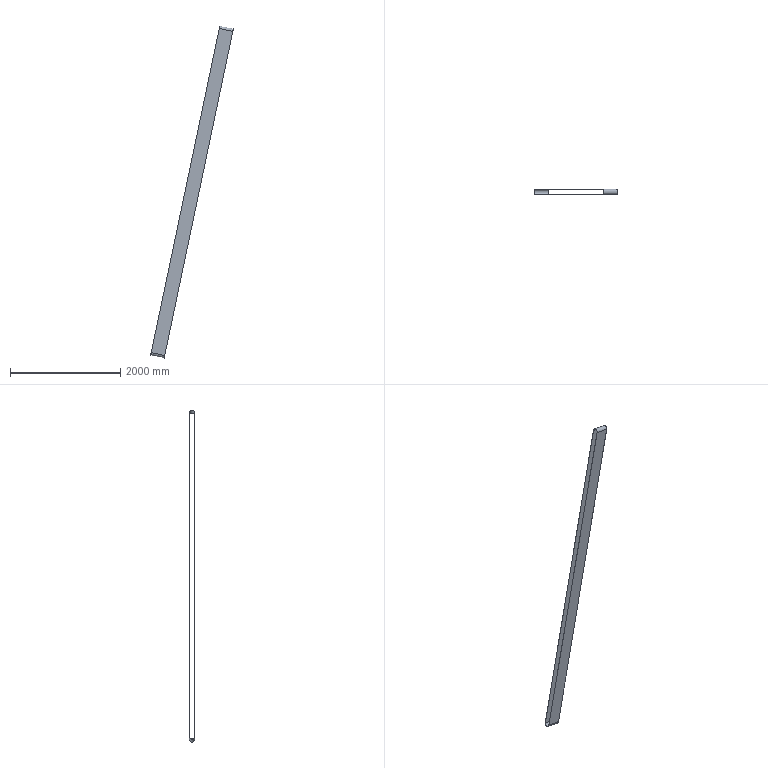Part | STEP file | ESTEIRA_003 | 1 solid | 10 faces | box 1498 x 95 x 6016 mm | volume 6146084 mm3 | plane 6 | cylinder 4 | commonest cylinder face diameters 91 x2 95 x2
STEP:
#1=CARTESIAN_POINT('',(0.,0.,0.));
#2=DIRECTION('',(0.,0.,1.));
#3=DIRECTION('',(1.,0.,0.));
#4=AXIS2_PLACEMENT_3D('',#1,#2,#3);
#5=CARTESIAN_POINT('',(-4261.561,-580.65,1712.598));
#6=VERTEX_POINT('',#5);
#7=CARTESIAN_POINT('',(-4506.218,-580.65,1764.008));
#8=VERTEX_POINT('',#7);
#9=CARTESIAN_POINT('',(-4261.561,-580.65,1712.598));
#10=DIRECTION('',(-0.9786,0.,0.2056));
#11=VECTOR('',#10,1.);
#12=LINE('',#9,#11);
#13=CARTESIAN_POINT('',(-4383.89,-580.65,1738.303));
#14=DIRECTION('',(0.,1.,0.));
#15=DIRECTION('',(0.,0.,1.));
#16=AXIS2_PLACEMENT_3D('',#13,#14,#15);
#17=PLANE('',#16);
#18=CARTESIAN_POINT('',(-25.705,122.328));
#19=DIRECTION('',(0.2056,-0.9786));
#20=VECTOR('',#19,1.);
#21=LINE('',#18,#20);
#22=(GEOMETRIC_REPRESENTATION_CONTEXT(2)PARAMETRIC_REPRESENTATION_CONTEXT()REPRESENTATION_CONTEXT('',''));
#23=DEFINITIONAL_REPRESENTATION('',(#21),#22);
#24=PCURVE('',#17,#23);
#25=CARTESIAN_POINT('',(-4383.89,-628.15,1738.303));
#26=DIRECTION('',(0.9786,0.,-0.2056));
#27=DIRECTION('',(0.,1.,0.));
#28=AXIS2_PLACEMENT_3D('',#25,#26,#27);
#29=CYLINDRICAL_SURFACE('',#28,47.5);
#30=CARTESIAN_POINT('',(0.,125.));
#31=DIRECTION('',(0.,-1.));
#32=VECTOR('',#31,1.);
#33=LINE('',#30,#32);
#34=(GEOMETRIC_REPRESENTATION_CONTEXT(2)PARAMETRIC_REPRESENTATION_CONTEXT()REPRESENTATION_CONTEXT('',''));
#35=DEFINITIONAL_REPRESENTATION('',(#33),#34);
#36=PCURVE('',#29,#35);
#37=SURFACE_CURVE('',#12,(#24,#36),.PCURVE_S1.);
#38=EDGE_CURVE('',#6,#8,#37,.T.);
#39=ORIENTED_EDGE('',*,*,#38,.F.);
#40=CARTESIAN_POINT('',(-5495.421,-580.65,-4159.165));
#41=VERTEX_POINT('',#40);
#42=CARTESIAN_POINT('',(-4261.561,-580.65,1712.598));
#43=DIRECTION('',(-0.2056,0.,-0.9786));
#44=VECTOR('',#43,1.);
#45=LINE('',#42,#44);
#46=CARTESIAN_POINT('',(-25.705,122.328));
#47=DIRECTION('',(-0.9786,-0.2056));
#48=VECTOR('',#47,1.);
#49=LINE('',#46,#48);
#50=(GEOMETRIC_REPRESENTATION_CONTEXT(2)PARAMETRIC_REPRESENTATION_CONTEXT()REPRESENTATION_CONTEXT('',''));
#51=DEFINITIONAL_REPRESENTATION('',(#49),#50);
#52=PCURVE('',#17,#51);
#53=CARTESIAN_POINT('',(-4426.,0.,930.055));
#54=DIRECTION('',(0.9786,0.,-0.2056));
#55=DIRECTION('',(-0.2056,0.,-0.9786));
#56=AXIS2_PLACEMENT_3D('',#53,#54,#55);
#57=PLANE('',#56);
#58=CARTESIAN_POINT('',(-799.633,-580.65));
#59=DIRECTION('',(1.,0.));
#60=VECTOR('',#59,1.);
#61=LINE('',#58,#60);
#62=(GEOMETRIC_REPRESENTATION_CONTEXT(2)PARAMETRIC_REPRESENTATION_CONTEXT()REPRESENTATION_CONTEXT('',''));
#63=DEFINITIONAL_REPRESENTATION('',(#61),#62);
#64=PCURVE('',#57,#63);
#65=SURFACE_CURVE('',#45,(#52,#64),.PCURVE_S1.);
#66=EDGE_CURVE('',#6,#41,#65,.T.);
#67=ORIENTED_EDGE('',*,*,#66,.T.);
#68=CARTESIAN_POINT('',(-5740.078,-580.65,-4107.754));
#69=VERTEX_POINT('',#68);
#70=CARTESIAN_POINT('',(-5495.421,-580.65,-4159.165));
#71=DIRECTION('',(-0.9786,0.,0.2056));
#72=VECTOR('',#71,1.);
#73=LINE('',#70,#72);
#74=CARTESIAN_POINT('',(-5897.468,-1111.531));
#75=DIRECTION('',(0.2056,-0.9786));
#76=VECTOR('',#75,1.);
#77=LINE('',#74,#76);
#78=(GEOMETRIC_REPRESENTATION_CONTEXT(2)PARAMETRIC_REPRESENTATION_CONTEXT()REPRESENTATION_CONTEXT('',''));
#79=DEFINITIONAL_REPRESENTATION('',(#77),#78);
#80=PCURVE('',#17,#79);
#81=CARTESIAN_POINT('',(-5617.749,-628.15,-4133.459));
#82=DIRECTION('',(0.9786,0.,-0.2056));
#83=DIRECTION('',(0.,-1.,0.));
#84=AXIS2_PLACEMENT_3D('',#81,#82,#83);
#85=CYLINDRICAL_SURFACE('',#84,47.5);
#86=CARTESIAN_POINT('',(3.142,125.));
#87=DIRECTION('',(0.,-1.));
#88=VECTOR('',#87,1.);
#89=LINE('',#86,#88);
#90=(GEOMETRIC_REPRESENTATION_CONTEXT(2)PARAMETRIC_REPRESENTATION_CONTEXT()REPRESENTATION_CONTEXT('',''));
#91=DEFINITIONAL_REPRESENTATION('',(#89),#90);
#92=PCURVE('',#85,#91);
#93=SURFACE_CURVE('',#73,(#80,#92),.PCURVE_S1.);
#94=EDGE_CURVE('',#41,#69,#93,.T.);
#95=ORIENTED_EDGE('',*,*,#94,.T.);
#96=CARTESIAN_POINT('',(-4506.218,-580.65,1764.008));
#97=DIRECTION('',(-0.2056,0.,-0.9786));
#98=VECTOR('',#97,1.);
#99=LINE('',#96,#98);
#100=CARTESIAN_POINT('',(25.705,-122.328));
#101=DIRECTION('',(-0.9786,-0.2056));
#102=VECTOR('',#101,1.);
#103=LINE('',#100,#102);
#104=(GEOMETRIC_REPRESENTATION_CONTEXT(2)PARAMETRIC_REPRESENTATION_CONTEXT()REPRESENTATION_CONTEXT('',''));
#105=DEFINITIONAL_REPRESENTATION('',(#103),#104);
#106=PCURVE('',#17,#105);
#107=CARTESIAN_POINT('',(-4670.657,0.,981.466));
#108=DIRECTION('',(0.9786,0.,-0.2056));
#109=DIRECTION('',(-0.2056,0.,-0.9786));
#110=AXIS2_PLACEMENT_3D('',#107,#108,#109);
#111=PLANE('',#110);
#112=CARTESIAN_POINT('',(-799.633,-580.65));
#113=DIRECTION('',(1.,0.));
#114=VECTOR('',#113,1.);
#115=LINE('',#112,#114);
#116=(GEOMETRIC_REPRESENTATION_CONTEXT(2)PARAMETRIC_REPRESENTATION_CONTEXT()REPRESENTATION_CONTEXT('',''));
#117=DEFINITIONAL_REPRESENTATION('',(#115),#116);
#118=PCURVE('',#111,#117);
#119=SURFACE_CURVE('',#99,(#106,#118),.PCURVE_S1.);
#120=EDGE_CURVE('',#8,#69,#119,.T.);
#121=ORIENTED_EDGE('',*,*,#120,.F.);
#122=EDGE_LOOP('',(#39,#67,#95,#121));
#123=FACE_BOUND('',#122,.T.);
#124=ADVANCED_FACE('',(#123),#17,.T.);
#125=CARTESIAN_POINT('',(-4506.218,-675.65,1764.008));
#126=VERTEX_POINT('',#125);
#127=CARTESIAN_POINT('',(-4506.218,-628.15,1764.008));
#128=DIRECTION('',(0.9786,0.,-0.2056));
#129=DIRECTION('',(0.2056,0.,0.9786));
#130=AXIS2_PLACEMENT_3D('',#127,#128,#129);
#131=CIRCLE('',#130,47.5);
#132=CARTESIAN_POINT('',(-4.712,-125.));
#133=DIRECTION('',(1.,0.));
#134=VECTOR('',#133,1.);
#135=LINE('',#132,#134);
#136=(GEOMETRIC_REPRESENTATION_CONTEXT(2)PARAMETRIC_REPRESENTATION_CONTEXT()REPRESENTATION_CONTEXT('',''));
#137=DEFINITIONAL_REPRESENTATION('',(#135),#136);
#138=PCURVE('',#29,#137);
#139=CARTESIAN_POINT('',(-799.633,-628.15));
#140=DIRECTION('',(-1.,0.));
#141=AXIS2_PLACEMENT_2D('',#139,#140);
#142=CIRCLE('',#141,47.5);
#143=(GEOMETRIC_REPRESENTATION_CONTEXT(2)PARAMETRIC_REPRESENTATION_CONTEXT()REPRESENTATION_CONTEXT('',''));
#144=DEFINITIONAL_REPRESENTATION('',(#142),#143);
#145=PCURVE('',#111,#144);
#146=SURFACE_CURVE('',#131,(#138,#145),.PCURVE_S1.);
#147=EDGE_CURVE('',#8,#126,#146,.T.);
#148=ORIENTED_EDGE('',*,*,#147,.T.);
#149=CARTESIAN_POINT('',(-4261.561,-675.65,1712.598));
#150=VERTEX_POINT('',#149);
#151=CARTESIAN_POINT('',(-4506.218,-675.65,1764.008));
#152=DIRECTION('',(0.9786,0.,-0.2056));
#153=VECTOR('',#152,1.);
#154=LINE('',#151,#153);
#155=CARTESIAN_POINT('',(3.142,-125.));
#156=DIRECTION('',(0.,1.));
#157=VECTOR('',#156,1.);
#158=LINE('',#155,#157);
#159=(GEOMETRIC_REPRESENTATION_CONTEXT(2)PARAMETRIC_REPRESENTATION_CONTEXT()REPRESENTATION_CONTEXT('',''));
#160=DEFINITIONAL_REPRESENTATION('',(#158),#159);
#161=PCURVE('',#29,#160);
#162=CARTESIAN_POINT('',(-5617.749,-675.65,-4133.459));
#163=DIRECTION('',(0.,-1.,0.));
#164=DIRECTION('',(0.,0.,-1.));
#165=AXIS2_PLACEMENT_3D('',#162,#163,#164);
#166=PLANE('',#165);
#167=CARTESIAN_POINT('',(-5897.468,1111.531));
#168=DIRECTION('',(0.2056,0.9786));
#169=VECTOR('',#168,1.);
#170=LINE('',#167,#169);
#171=(GEOMETRIC_REPRESENTATION_CONTEXT(2)PARAMETRIC_REPRESENTATION_CONTEXT()REPRESENTATION_CONTEXT('',''));
#172=DEFINITIONAL_REPRESENTATION('',(#170),#171);
#173=PCURVE('',#166,#172);
#174=SURFACE_CURVE('',#154,(#161,#173),.PCURVE_S1.);
#175=EDGE_CURVE('',#126,#150,#174,.T.);
#176=ORIENTED_EDGE('',*,*,#175,.T.);
#177=CARTESIAN_POINT('',(-4261.561,-628.15,1712.598));
#178=DIRECTION('',(0.9786,0.,-0.2056));
#179=DIRECTION('',(0.2056,0.,0.9786));
#180=AXIS2_PLACEMENT_3D('',#177,#178,#179);
#181=CIRCLE('',#180,47.5);
#182=CARTESIAN_POINT('',(-4.712,125.));
#183=DIRECTION('',(1.,0.));
#184=VECTOR('',#183,1.);
#185=LINE('',#182,#184);
#186=(GEOMETRIC_REPRESENTATION_CONTEXT(2)PARAMETRIC_REPRESENTATION_CONTEXT()REPRESENTATION_CONTEXT('',''));
#187=DEFINITIONAL_REPRESENTATION('',(#185),#186);
#188=PCURVE('',#29,#187);
#189=CARTESIAN_POINT('',(-799.633,-628.15));
#190=DIRECTION('',(-1.,0.));
#191=AXIS2_PLACEMENT_2D('',#189,#190);
#192=CIRCLE('',#191,47.5);
#193=(GEOMETRIC_REPRESENTATION_CONTEXT(2)PARAMETRIC_REPRESENTATION_CONTEXT()REPRESENTATION_CONTEXT('',''));
#194=DEFINITIONAL_REPRESENTATION('',(#192),#193);
#195=PCURVE('',#57,#194);
#196=SURFACE_CURVE('',#181,(#188,#195),.PCURVE_S1.);
#197=EDGE_CURVE('',#6,#150,#196,.T.);
#198=ORIENTED_EDGE('',*,*,#197,.F.);
#199=ORIENTED_EDGE('',*,*,#38,.T.);
#200=EDGE_LOOP('',(#148,#176,#198,#199));
#201=FACE_BOUND('',#200,.T.);
#202=ADVANCED_FACE('',(#201),#29,.T.);
#203=CARTESIAN_POINT('',(-5495.421,-675.65,-4159.165));
#204=VERTEX_POINT('',#203);
#205=CARTESIAN_POINT('',(-5740.078,-675.65,-4107.754));
#206=VERTEX_POINT('',#205);
#207=CARTESIAN_POINT('',(-5495.421,-675.65,-4159.165));
#208=DIRECTION('',(-0.9786,0.,0.2056));
#209=VECTOR('',#208,1.);
#210=LINE('',#207,#209);
#211=CARTESIAN_POINT('',(25.705,122.328));
#212=DIRECTION('',(-0.2056,-0.9786));
#213=VECTOR('',#212,1.);
#214=LINE('',#211,#213);
#215=(GEOMETRIC_REPRESENTATION_CONTEXT(2)PARAMETRIC_REPRESENTATION_CONTEXT()REPRESENTATION_CONTEXT('',''));
#216=DEFINITIONAL_REPRESENTATION('',(#214),#215);
#217=PCURVE('',#166,#216);
#218=CARTESIAN_POINT('',(0.,125.));
#219=DIRECTION('',(0.,-1.));
#220=VECTOR('',#219,1.);
#221=LINE('',#218,#220);
#222=(GEOMETRIC_REPRESENTATION_CONTEXT(2)PARAMETRIC_REPRESENTATION_CONTEXT()REPRESENTATION_CONTEXT('',''));
#223=DEFINITIONAL_REPRESENTATION('',(#221),#222);
#224=PCURVE('',#85,#223);
#225=SURFACE_CURVE('',#210,(#217,#224),.PCURVE_S1.);
#226=EDGE_CURVE('',#204,#206,#225,.T.);
#227=ORIENTED_EDGE('',*,*,#226,.F.);
#228=CARTESIAN_POINT('',(-5495.421,-675.65,-4159.165));
#229=DIRECTION('',(0.2056,0.,0.9786));
#230=VECTOR('',#229,1.);
#231=LINE('',#228,#230);
#232=CARTESIAN_POINT('',(25.705,122.328));
#233=DIRECTION('',(-0.9786,0.2056));
#234=VECTOR('',#233,1.);
#235=LINE('',#232,#234);
#236=(GEOMETRIC_REPRESENTATION_CONTEXT(2)PARAMETRIC_REPRESENTATION_CONTEXT()REPRESENTATION_CONTEXT('',''));
#237=DEFINITIONAL_REPRESENTATION('',(#235),#236);
#238=PCURVE('',#166,#237);
#239=CARTESIAN_POINT('',(5200.367,-675.65));
#240=DIRECTION('',(-1.,0.));
#241=VECTOR('',#240,1.);
#242=LINE('',#239,#241);
#243=(GEOMETRIC_REPRESENTATION_CONTEXT(2)PARAMETRIC_REPRESENTATION_CONTEXT()REPRESENTATION_CONTEXT('',''));
#244=DEFINITIONAL_REPRESENTATION('',(#242),#243);
#245=PCURVE('',#57,#244);
#246=SURFACE_CURVE('',#231,(#238,#245),.PCURVE_S1.);
#247=EDGE_CURVE('',#204,#150,#246,.T.);
#248=ORIENTED_EDGE('',*,*,#247,.T.);
#249=ORIENTED_EDGE('',*,*,#175,.F.);
#250=CARTESIAN_POINT('',(-5740.078,-675.65,-4107.754));
#251=DIRECTION('',(0.2056,0.,0.9786));
#252=VECTOR('',#251,1.);
#253=LINE('',#250,#252);
#254=CARTESIAN_POINT('',(-25.705,-122.328));
#255=DIRECTION('',(-0.9786,0.2056));
#256=VECTOR('',#255,1.);
#257=LINE('',#254,#256);
#258=(GEOMETRIC_REPRESENTATION_CONTEXT(2)PARAMETRIC_REPRESENTATION_CONTEXT()REPRESENTATION_CONTEXT('',''));
#259=DEFINITIONAL_REPRESENTATION('',(#257),#258);
#260=PCURVE('',#166,#259);
#261=CARTESIAN_POINT('',(5200.367,-675.65));
#262=DIRECTION('',(-1.,0.));
#263=VECTOR('',#262,1.);
#264=LINE('',#261,#263);
#265=(GEOMETRIC_REPRESENTATION_CONTEXT(2)PARAMETRIC_REPRESENTATION_CONTEXT()REPRESENTATION_CONTEXT('',''));
#266=DEFINITIONAL_REPRESENTATION('',(#264),#265);
#267=PCURVE('',#111,#266);
#268=SURFACE_CURVE('',#253,(#260,#267),.PCURVE_S1.);
#269=EDGE_CURVE('',#206,#126,#268,.T.);
#270=ORIENTED_EDGE('',*,*,#269,.F.);
#271=EDGE_LOOP('',(#227,#248,#249,#270));
#272=FACE_BOUND('',#271,.T.);
#273=ADVANCED_FACE('',(#272),#166,.T.);
#274=CARTESIAN_POINT('',(-5740.078,-628.15,-4107.754));
#275=DIRECTION('',(0.9786,0.,-0.2056));
#276=DIRECTION('',(0.2056,0.,0.9786));
#277=AXIS2_PLACEMENT_3D('',#274,#275,#276);
#278=CIRCLE('',#277,47.5);
#279=CARTESIAN_POINT('',(-1.571,-125.));
#280=DIRECTION('',(1.,0.));
#281=VECTOR('',#280,1.);
#282=LINE('',#279,#281);
#283=(GEOMETRIC_REPRESENTATION_CONTEXT(2)PARAMETRIC_REPRESENTATION_CONTEXT()REPRESENTATION_CONTEXT('',''));
#284=DEFINITIONAL_REPRESENTATION('',(#282),#283);
#285=PCURVE('',#85,#284);
#286=CARTESIAN_POINT('',(5200.367,-628.15));
#287=DIRECTION('',(-1.,0.));
#288=AXIS2_PLACEMENT_2D('',#286,#287);
#289=CIRCLE('',#288,47.5);
#290=(GEOMETRIC_REPRESENTATION_CONTEXT(2)PARAMETRIC_REPRESENTATION_CONTEXT()REPRESENTATION_CONTEXT('',''));
#291=DEFINITIONAL_REPRESENTATION('',(#289),#290);
#292=PCURVE('',#111,#291);
#293=SURFACE_CURVE('',#278,(#285,#292),.PCURVE_S1.);
#294=EDGE_CURVE('',#206,#69,#293,.T.);
#295=ORIENTED_EDGE('',*,*,#294,.T.);
#296=ORIENTED_EDGE('',*,*,#94,.F.);
#297=CARTESIAN_POINT('',(-5495.421,-628.15,-4159.165));
#298=DIRECTION('',(0.9786,0.,-0.2056));
#299=DIRECTION('',(0.2056,0.,0.9786));
#300=AXIS2_PLACEMENT_3D('',#297,#298,#299);
#301=CIRCLE('',#300,47.5);
#302=CARTESIAN_POINT('',(-1.571,125.));
#303=DIRECTION('',(1.,0.));
#304=VECTOR('',#303,1.);
#305=LINE('',#302,#304);
#306=(GEOMETRIC_REPRESENTATION_CONTEXT(2)PARAMETRIC_REPRESENTATION_CONTEXT()REPRESENTATION_CONTEXT('',''));
#307=DEFINITIONAL_REPRESENTATION('',(#305),#306);
#308=PCURVE('',#85,#307);
#309=CARTESIAN_POINT('',(5200.367,-628.15));
#310=DIRECTION('',(-1.,0.));
#311=AXIS2_PLACEMENT_2D('',#309,#310);
#312=CIRCLE('',#311,47.5);
#313=(GEOMETRIC_REPRESENTATION_CONTEXT(2)PARAMETRIC_REPRESENTATION_CONTEXT()REPRESENTATION_CONTEXT('',''));
#314=DEFINITIONAL_REPRESENTATION('',(#312),#313);
#315=PCURVE('',#57,#314);
#316=SURFACE_CURVE('',#301,(#308,#315),.PCURVE_S1.);
#317=EDGE_CURVE('',#204,#41,#316,.T.);
#318=ORIENTED_EDGE('',*,*,#317,.F.);
#319=ORIENTED_EDGE('',*,*,#226,.T.);
#320=EDGE_LOOP('',(#295,#296,#318,#319));
#321=FACE_BOUND('',#320,.T.);
#322=ADVANCED_FACE('',(#321),#85,.T.);
#323=CARTESIAN_POINT('',(-4506.218,-582.65,1764.008));
#324=VERTEX_POINT('',#323);
#325=CARTESIAN_POINT('',(-5740.078,-582.65,-4107.754));
#326=VERTEX_POINT('',#325);
#327=CARTESIAN_POINT('',(-4506.218,-582.65,1764.008));
#328=DIRECTION('',(-0.2056,0.,-0.9786));
#329=VECTOR('',#328,1.);
#330=LINE('',#327,#329);
#331=CARTESIAN_POINT('',(-4383.89,-582.65,1738.303));
#332=DIRECTION('',(0.,1.,0.));
#333=DIRECTION('',(0.,0.,1.));
#334=AXIS2_PLACEMENT_3D('',#331,#332,#333);
#335=PLANE('',#334);
#336=CARTESIAN_POINT('',(25.705,-122.328));
#337=DIRECTION('',(-0.9786,-0.2056));
#338=VECTOR('',#337,1.);
#339=LINE('',#336,#338);
#340=(GEOMETRIC_REPRESENTATION_CONTEXT(2)PARAMETRIC_REPRESENTATION_CONTEXT()REPRESENTATION_CONTEXT('',''));
#341=DEFINITIONAL_REPRESENTATION('',(#339),#340);
#342=PCURVE('',#335,#341);
#343=CARTESIAN_POINT('',(-799.633,-582.65));
#344=DIRECTION('',(1.,0.));
#345=VECTOR('',#344,1.);
#346=LINE('',#343,#345);
#347=(GEOMETRIC_REPRESENTATION_CONTEXT(2)PARAMETRIC_REPRESENTATION_CONTEXT()REPRESENTATION_CONTEXT('',''));
#348=DEFINITIONAL_REPRESENTATION('',(#346),#347);
#349=PCURVE('',#111,#348);
#350=SURFACE_CURVE('',#330,(#342,#349),.PCURVE_S1.);
#351=EDGE_CURVE('',#324,#326,#350,.T.);
#352=ORIENTED_EDGE('',*,*,#351,.T.);
#353=CARTESIAN_POINT('',(-5495.421,-582.65,-4159.165));
#354=VERTEX_POINT('',#353);
#355=CARTESIAN_POINT('',(-5495.421,-582.65,-4159.165));
#356=DIRECTION('',(-0.9786,0.,0.2056));
#357=VECTOR('',#356,1.);
#358=LINE('',#355,#357);
#359=CARTESIAN_POINT('',(-5897.468,-1111.531));
#360=DIRECTION('',(0.2056,-0.9786));
#361=VECTOR('',#360,1.);
#362=LINE('',#359,#361);
#363=(GEOMETRIC_REPRESENTATION_CONTEXT(2)PARAMETRIC_REPRESENTATION_CONTEXT()REPRESENTATION_CONTEXT('',''));
#364=DEFINITIONAL_REPRESENTATION('',(#362),#363);
#365=PCURVE('',#335,#364);
#366=CARTESIAN_POINT('',(-5617.749,-628.15,-4133.459));
#367=DIRECTION('',(0.9786,0.,-0.2056));
#368=DIRECTION('',(0.,-1.,0.));
#369=AXIS2_PLACEMENT_3D('',#366,#367,#368);
#370=CYLINDRICAL_SURFACE('',#369,45.5);
#371=CARTESIAN_POINT('',(3.142,125.));
#372=DIRECTION('',(0.,-1.));
#373=VECTOR('',#372,1.);
#374=LINE('',#371,#373);
#375=(GEOMETRIC_REPRESENTATION_CONTEXT(2)PARAMETRIC_REPRESENTATION_CONTEXT()REPRESENTATION_CONTEXT('',''));
#376=DEFINITIONAL_REPRESENTATION('',(#374),#375);
#377=PCURVE('',#370,#376);
#378=SURFACE_CURVE('',#358,(#365,#377),.PCURVE_S1.);
#379=EDGE_CURVE('',#354,#326,#378,.T.);
#380=ORIENTED_EDGE('',*,*,#379,.F.);
#381=CARTESIAN_POINT('',(-4261.561,-582.65,1712.598));
#382=VERTEX_POINT('',#381);
#383=CARTESIAN_POINT('',(-4261.561,-582.65,1712.598));
#384=DIRECTION('',(-0.2056,0.,-0.9786));
#385=VECTOR('',#384,1.);
#386=LINE('',#383,#385);
#387=CARTESIAN_POINT('',(-25.705,122.328));
#388=DIRECTION('',(-0.9786,-0.2056));
#389=VECTOR('',#388,1.);
#390=LINE('',#387,#389);
#391=(GEOMETRIC_REPRESENTATION_CONTEXT(2)PARAMETRIC_REPRESENTATION_CONTEXT()REPRESENTATION_CONTEXT('',''));
#392=DEFINITIONAL_REPRESENTATION('',(#390),#391);
#393=PCURVE('',#335,#392);
#394=CARTESIAN_POINT('',(-799.633,-582.65));
#395=DIRECTION('',(1.,0.));
#396=VECTOR('',#395,1.);
#397=LINE('',#394,#396);
#398=(GEOMETRIC_REPRESENTATION_CONTEXT(2)PARAMETRIC_REPRESENTATION_CONTEXT()REPRESENTATION_CONTEXT('',''));
#399=DEFINITIONAL_REPRESENTATION('',(#397),#398);
#400=PCURVE('',#57,#399);
#401=SURFACE_CURVE('',#386,(#393,#400),.PCURVE_S1.);
#402=EDGE_CURVE('',#382,#354,#401,.T.);
#403=ORIENTED_EDGE('',*,*,#402,.F.);
#404=CARTESIAN_POINT('',(-4261.561,-582.65,1712.598));
#405=DIRECTION('',(-0.9786,0.,0.2056));
#406=VECTOR('',#405,1.);
#407=LINE('',#404,#406);
#408=CARTESIAN_POINT('',(-25.705,122.328));
#409=DIRECTION('',(0.2056,-0.9786));
#410=VECTOR('',#409,1.);
#411=LINE('',#408,#410);
#412=(GEOMETRIC_REPRESENTATION_CONTEXT(2)PARAMETRIC_REPRESENTATION_CONTEXT()REPRESENTATION_CONTEXT('',''));
#413=DEFINITIONAL_REPRESENTATION('',(#411),#412);
#414=PCURVE('',#335,#413);
#415=CARTESIAN_POINT('',(-4383.89,-628.15,1738.303));
#416=DIRECTION('',(0.9786,0.,-0.2056));
#417=DIRECTION('',(0.,1.,0.));
#418=AXIS2_PLACEMENT_3D('',#415,#416,#417);
#419=CYLINDRICAL_SURFACE('',#418,45.5);
#420=CARTESIAN_POINT('',(0.,125.));
#421=DIRECTION('',(0.,-1.));
#422=VECTOR('',#421,1.);
#423=LINE('',#420,#422);
#424=(GEOMETRIC_REPRESENTATION_CONTEXT(2)PARAMETRIC_REPRESENTATION_CONTEXT()REPRESENTATION_CONTEXT('',''));
#425=DEFINITIONAL_REPRESENTATION('',(#423),#424);
#426=PCURVE('',#419,#425);
#427=SURFACE_CURVE('',#407,(#414,#426),.PCURVE_S1.);
#428=EDGE_CURVE('',#382,#324,#427,.T.);
#429=ORIENTED_EDGE('',*,*,#428,.T.);
#430=EDGE_LOOP('',(#352,#380,#403,#429));
#431=FACE_BOUND('',#430,.T.);
#432=ADVANCED_FACE('',(#431),#335,.F.);
#433=CARTESIAN_POINT('',(-5740.078,-673.65,-4107.754));
#434=VERTEX_POINT('',#433);
#435=CARTESIAN_POINT('',(-5740.078,-628.15,-4107.754));
#436=DIRECTION('',(0.9786,0.,-0.2056));
#437=DIRECTION('',(0.2056,0.,0.9786));
#438=AXIS2_PLACEMENT_3D('',#435,#436,#437);
#439=CIRCLE('',#438,45.5);
#440=CARTESIAN_POINT('',(-1.571,-125.));
#441=DIRECTION('',(1.,0.));
#442=VECTOR('',#441,1.);
#443=LINE('',#440,#442);
#444=(GEOMETRIC_REPRESENTATION_CONTEXT(2)PARAMETRIC_REPRESENTATION_CONTEXT()REPRESENTATION_CONTEXT('',''));
#445=DEFINITIONAL_REPRESENTATION('',(#443),#444);
#446=PCURVE('',#370,#445);
#447=CARTESIAN_POINT('',(5200.367,-628.15));
#448=DIRECTION('',(-1.,0.));
#449=AXIS2_PLACEMENT_2D('',#447,#448);
#450=CIRCLE('',#449,45.5);
#451=(GEOMETRIC_REPRESENTATION_CONTEXT(2)PARAMETRIC_REPRESENTATION_CONTEXT()REPRESENTATION_CONTEXT('',''));
#452=DEFINITIONAL_REPRESENTATION('',(#450),#451);
#453=PCURVE('',#111,#452);
#454=SURFACE_CURVE('',#439,(#446,#453),.PCURVE_S1.);
#455=EDGE_CURVE('',#434,#326,#454,.T.);
#456=ORIENTED_EDGE('',*,*,#455,.T.);
#457=ORIENTED_EDGE('',*,*,#379,.F.);
#458=CARTESIAN_POINT('',(-5495.421,-673.65,-4159.165));
#459=VERTEX_POINT('',#458);
#460=CARTESIAN_POINT('',(-5495.421,-628.15,-4159.165));
#461=DIRECTION('',(0.9786,0.,-0.2056));
#462=DIRECTION('',(0.2056,0.,0.9786));
#463=AXIS2_PLACEMENT_3D('',#460,#461,#462);
#464=CIRCLE('',#463,45.5);
#465=CARTESIAN_POINT('',(-1.571,125.));
#466=DIRECTION('',(1.,0.));
#467=VECTOR('',#466,1.);
#468=LINE('',#465,#467);
#469=(GEOMETRIC_REPRESENTATION_CONTEXT(2)PARAMETRIC_REPRESENTATION_CONTEXT()REPRESENTATION_CONTEXT('',''));
#470=DEFINITIONAL_REPRESENTATION('',(#468),#469);
#471=PCURVE('',#370,#470);
#472=CARTESIAN_POINT('',(5200.367,-628.15));
#473=DIRECTION('',(-1.,0.));
#474=AXIS2_PLACEMENT_2D('',#472,#473);
#475=CIRCLE('',#474,45.5);
#476=(GEOMETRIC_REPRESENTATION_CONTEXT(2)PARAMETRIC_REPRESENTATION_CONTEXT()REPRESENTATION_CONTEXT('',''));
#477=DEFINITIONAL_REPRESENTATION('',(#475),#476);
#478=PCURVE('',#57,#477);
#479=SURFACE_CURVE('',#464,(#471,#478),.PCURVE_S1.);
#480=EDGE_CURVE('',#459,#354,#479,.T.);
#481=ORIENTED_EDGE('',*,*,#480,.F.);
#482=CARTESIAN_POINT('',(-5740.078,-673.65,-4107.754));
#483=DIRECTION('',(0.9786,0.,-0.2056));
#484=VECTOR('',#483,1.);
#485=LINE('',#482,#484);
#486=CARTESIAN_POINT('',(0.,-125.));
#487=DIRECTION('',(0.,1.));
#488=VECTOR('',#487,1.);
#489=LINE('',#486,#488);
#490=(GEOMETRIC_REPRESENTATION_CONTEXT(2)PARAMETRIC_REPRESENTATION_CONTEXT()REPRESENTATION_CONTEXT('',''));
#491=DEFINITIONAL_REPRESENTATION('',(#489),#490);
#492=PCURVE('',#370,#491);
#493=CARTESIAN_POINT('',(-5617.749,-673.65,-4133.459));
#494=DIRECTION('',(0.,-1.,0.));
#495=DIRECTION('',(0.,0.,-1.));
#496=AXIS2_PLACEMENT_3D('',#493,#494,#495);
#497=PLANE('',#496);
#498=CARTESIAN_POINT('',(-25.705,-122.328));
#499=DIRECTION('',(0.2056,0.9786));
#500=VECTOR('',#499,1.);
#501=LINE('',#498,#500);
#502=(GEOMETRIC_REPRESENTATION_CONTEXT(2)PARAMETRIC_REPRESENTATION_CONTEXT()REPRESENTATION_CONTEXT('',''));
#503=DEFINITIONAL_REPRESENTATION('',(#501),#502);
#504=PCURVE('',#497,#503);
#505=SURFACE_CURVE('',#485,(#492,#504),.PCURVE_S1.);
#506=EDGE_CURVE('',#434,#459,#505,.T.);
#507=ORIENTED_EDGE('',*,*,#506,.F.);
#508=EDGE_LOOP('',(#456,#457,#481,#507));
#509=FACE_BOUND('',#508,.F.);
#510=ADVANCED_FACE('',(#509),#370,.F.);
#511=CARTESIAN_POINT('',(-4506.218,-673.65,1764.008));
#512=VERTEX_POINT('',#511);
#513=CARTESIAN_POINT('',(-5740.078,-673.65,-4107.754));
#514=DIRECTION('',(0.2056,0.,0.9786));
#515=VECTOR('',#514,1.);
#516=LINE('',#513,#515);
#517=CARTESIAN_POINT('',(-25.705,-122.328));
#518=DIRECTION('',(-0.9786,0.2056));
#519=VECTOR('',#518,1.);
#520=LINE('',#517,#519);
#521=(GEOMETRIC_REPRESENTATION_CONTEXT(2)PARAMETRIC_REPRESENTATION_CONTEXT()REPRESENTATION_CONTEXT('',''));
#522=DEFINITIONAL_REPRESENTATION('',(#520),#521);
#523=PCURVE('',#497,#522);
#524=CARTESIAN_POINT('',(5200.367,-673.65));
#525=DIRECTION('',(-1.,0.));
#526=VECTOR('',#525,1.);
#527=LINE('',#524,#526);
#528=(GEOMETRIC_REPRESENTATION_CONTEXT(2)PARAMETRIC_REPRESENTATION_CONTEXT()REPRESENTATION_CONTEXT('',''));
#529=DEFINITIONAL_REPRESENTATION('',(#527),#528);
#530=PCURVE('',#111,#529);
#531=SURFACE_CURVE('',#516,(#523,#530),.PCURVE_S1.);
#532=EDGE_CURVE('',#434,#512,#531,.T.);
#533=ORIENTED_EDGE('',*,*,#532,.T.);
#534=CARTESIAN_POINT('',(-4261.561,-673.65,1712.598));
#535=VERTEX_POINT('',#534);
#536=CARTESIAN_POINT('',(-4261.561,-673.65,1712.598));
#537=DIRECTION('',(-0.9786,0.,0.2056));
#538=VECTOR('',#537,1.);
#539=LINE('',#536,#538);
#540=CARTESIAN_POINT('',(-5846.057,1356.188));
#541=DIRECTION('',(-0.2056,-0.9786));
#542=VECTOR('',#541,1.);
#543=LINE('',#540,#542);
#544=(GEOMETRIC_REPRESENTATION_CONTEXT(2)PARAMETRIC_REPRESENTATION_CONTEXT()REPRESENTATION_CONTEXT('',''));
#545=DEFINITIONAL_REPRESENTATION('',(#543),#544);
#546=PCURVE('',#497,#545);
#547=CARTESIAN_POINT('',(3.142,125.));
#548=DIRECTION('',(0.,-1.));
#549=VECTOR('',#548,1.);
#550=LINE('',#547,#549);
#551=(GEOMETRIC_REPRESENTATION_CONTEXT(2)PARAMETRIC_REPRESENTATION_CONTEXT()REPRESENTATION_CONTEXT('',''));
#552=DEFINITIONAL_REPRESENTATION('',(#550),#551);
#553=PCURVE('',#419,#552);
#554=SURFACE_CURVE('',#539,(#546,#553),.PCURVE_S1.);
#555=EDGE_CURVE('',#535,#512,#554,.T.);
#556=ORIENTED_EDGE('',*,*,#555,.F.);
#557=CARTESIAN_POINT('',(-5495.421,-673.65,-4159.165));
#558=DIRECTION('',(0.2056,0.,0.9786));
#559=VECTOR('',#558,1.);
#560=LINE('',#557,#559);
#561=CARTESIAN_POINT('',(25.705,122.328));
#562=DIRECTION('',(-0.9786,0.2056));
#563=VECTOR('',#562,1.);
#564=LINE('',#561,#563);
#565=(GEOMETRIC_REPRESENTATION_CONTEXT(2)PARAMETRIC_REPRESENTATION_CONTEXT()REPRESENTATION_CONTEXT('',''));
#566=DEFINITIONAL_REPRESENTATION('',(#564),#565);
#567=PCURVE('',#497,#566);
#568=CARTESIAN_POINT('',(5200.367,-673.65));
#569=DIRECTION('',(-1.,0.));
#570=VECTOR('',#569,1.);
#571=LINE('',#568,#570);
#572=(GEOMETRIC_REPRESENTATION_CONTEXT(2)PARAMETRIC_REPRESENTATION_CONTEXT()REPRESENTATION_CONTEXT('',''));
#573=DEFINITIONAL_REPRESENTATION('',(#571),#572);
#574=PCURVE('',#57,#573);
#575=SURFACE_CURVE('',#560,(#567,#574),.PCURVE_S1.);
#576=EDGE_CURVE('',#459,#535,#575,.T.);
#577=ORIENTED_EDGE('',*,*,#576,.F.);
#578=ORIENTED_EDGE('',*,*,#506,.F.);
#579=EDGE_LOOP('',(#533,#556,#577,#578));
#580=FACE_BOUND('',#579,.T.);
#581=ADVANCED_FACE('',(#580),#497,.F.);
#582=CARTESIAN_POINT('',(-4506.218,-628.15,1764.008));
#583=DIRECTION('',(0.9786,0.,-0.2056));
#584=DIRECTION('',(0.2056,0.,0.9786));
#585=AXIS2_PLACEMENT_3D('',#582,#583,#584);
#586=CIRCLE('',#585,45.5);
#587=CARTESIAN_POINT('',(-4.712,-125.));
#588=DIRECTION('',(1.,0.));
#589=VECTOR('',#588,1.);
#590=LINE('',#587,#589);
#591=(GEOMETRIC_REPRESENTATION_CONTEXT(2)PARAMETRIC_REPRESENTATION_CONTEXT()REPRESENTATION_CONTEXT('',''));
#592=DEFINITIONAL_REPRESENTATION('',(#590),#591);
#593=PCURVE('',#419,#592);
#594=CARTESIAN_POINT('',(-799.633,-628.15));
#595=DIRECTION('',(-1.,0.));
#596=AXIS2_PLACEMENT_2D('',#594,#595);
#597=CIRCLE('',#596,45.5);
#598=(GEOMETRIC_REPRESENTATION_CONTEXT(2)PARAMETRIC_REPRESENTATION_CONTEXT()REPRESENTATION_CONTEXT('',''));
#599=DEFINITIONAL_REPRESENTATION('',(#597),#598);
#600=PCURVE('',#111,#599);
#601=SURFACE_CURVE('',#586,(#593,#600),.PCURVE_S1.);
#602=EDGE_CURVE('',#324,#512,#601,.T.);
#603=ORIENTED_EDGE('',*,*,#602,.T.);
#604=ORIENTED_EDGE('',*,*,#555,.F.);
#605=CARTESIAN_POINT('',(-4261.561,-628.15,1712.598));
#606=DIRECTION('',(0.9786,0.,-0.2056));
#607=DIRECTION('',(0.2056,0.,0.9786));
#608=AXIS2_PLACEMENT_3D('',#605,#606,#607);
#609=CIRCLE('',#608,45.5);
#610=CARTESIAN_POINT('',(-4.712,125.));
#611=DIRECTION('',(1.,0.));
#612=VECTOR('',#611,1.);
#613=LINE('',#610,#612);
#614=(GEOMETRIC_REPRESENTATION_CONTEXT(2)PARAMETRIC_REPRESENTATION_CONTEXT()REPRESENTATION_CONTEXT('',''));
#615=DEFINITIONAL_REPRESENTATION('',(#613),#614);
#616=PCURVE('',#419,#615);
#617=CARTESIAN_POINT('',(-799.633,-628.15));
#618=DIRECTION('',(-1.,0.));
#619=AXIS2_PLACEMENT_2D('',#617,#618);
#620=CIRCLE('',#619,45.5);
#621=(GEOMETRIC_REPRESENTATION_CONTEXT(2)PARAMETRIC_REPRESENTATION_CONTEXT()REPRESENTATION_CONTEXT('',''));
#622=DEFINITIONAL_REPRESENTATION('',(#620),#621);
#623=PCURVE('',#57,#622);
#624=SURFACE_CURVE('',#609,(#616,#623),.PCURVE_S1.);
#625=EDGE_CURVE('',#382,#535,#624,.T.);
#626=ORIENTED_EDGE('',*,*,#625,.F.);
#627=ORIENTED_EDGE('',*,*,#428,.T.);
#628=EDGE_LOOP('',(#603,#604,#626,#627));
#629=FACE_BOUND('',#628,.F.);
#630=ADVANCED_FACE('',(#629),#419,.F.);
#631=ORIENTED_EDGE('',*,*,#66,.F.);
#632=ORIENTED_EDGE('',*,*,#197,.T.);
#633=ORIENTED_EDGE('',*,*,#247,.F.);
#634=ORIENTED_EDGE('',*,*,#317,.T.);
#635=EDGE_LOOP('',(#631,#632,#633,#634));
#636=FACE_BOUND('',#635,.T.);
#637=ORIENTED_EDGE('',*,*,#402,.T.);
#638=ORIENTED_EDGE('',*,*,#480,.F.);
#639=ORIENTED_EDGE('',*,*,#576,.T.);
#640=ORIENTED_EDGE('',*,*,#625,.F.);
#641=EDGE_LOOP('',(#637,#638,#639,#640));
#642=FACE_BOUND('',#641,.T.);
#643=ADVANCED_FACE('',(#636,#642),#57,.T.);
#644=ORIENTED_EDGE('',*,*,#294,.F.);
#645=ORIENTED_EDGE('',*,*,#269,.T.);
#646=ORIENTED_EDGE('',*,*,#147,.F.);
#647=ORIENTED_EDGE('',*,*,#120,.T.);
#648=EDGE_LOOP('',(#644,#645,#646,#647));
#649=FACE_BOUND('',#648,.T.);
#650=ORIENTED_EDGE('',*,*,#602,.T.);
#651=ORIENTED_EDGE('',*,*,#532,.F.);
#652=ORIENTED_EDGE('',*,*,#455,.T.);
#653=ORIENTED_EDGE('',*,*,#351,.F.);
#654=EDGE_LOOP('',(#650,#651,#652,#653));
#655=FACE_BOUND('',#654,.T.);
#656=ADVANCED_FACE('',(#649,#655),#111,.F.);
#657=CLOSED_SHELL('',(#124,#202,#273,#322,#432,#510,#581,#630,#643,#656));
#658=MANIFOLD_SOLID_BREP('',#657);
#659=(LENGTH_UNIT()NAMED_UNIT(*)SI_UNIT(.MILLI.,.METRE.));
#660=UNCERTAINTY_MEASURE_WITH_UNIT(LENGTH_MEASURE(0.0000001),#659,'','');
#661=(NAMED_UNIT(*)PLANE_ANGLE_UNIT()SI_UNIT($,.RADIAN.));
#662=(NAMED_UNIT(*)SI_UNIT($,.STERADIAN.)SOLID_ANGLE_UNIT());
#663=(GEOMETRIC_REPRESENTATION_CONTEXT(3)GLOBAL_UNCERTAINTY_ASSIGNED_CONTEXT((#660))GLOBAL_UNIT_ASSIGNED_CONTEXT((#659,#661,#662))REPRESENTATION_CONTEXT('',''));
#664=ADVANCED_BREP_SHAPE_REPRESENTATION('',(#4,#658),#663);